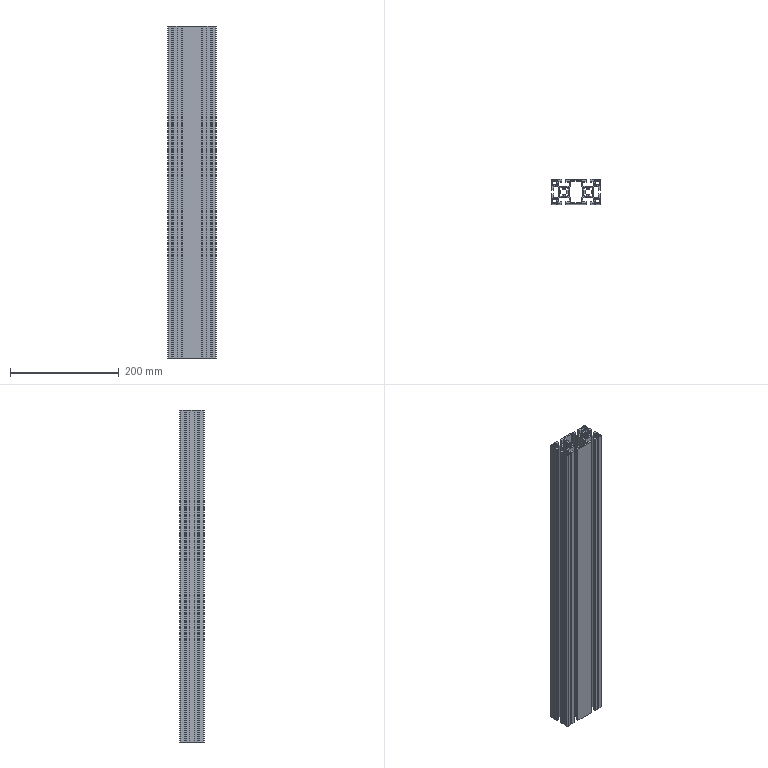Part | STEP file | 4590-600 Al (base long) | 1 solid | 366 faces | box 90 x 45 x 610 mm | volume 715349 mm3 | plane 254 | cylinder 112 | commonest cylinder face diameters 2 x64 8 x20 12 x16 4 x12